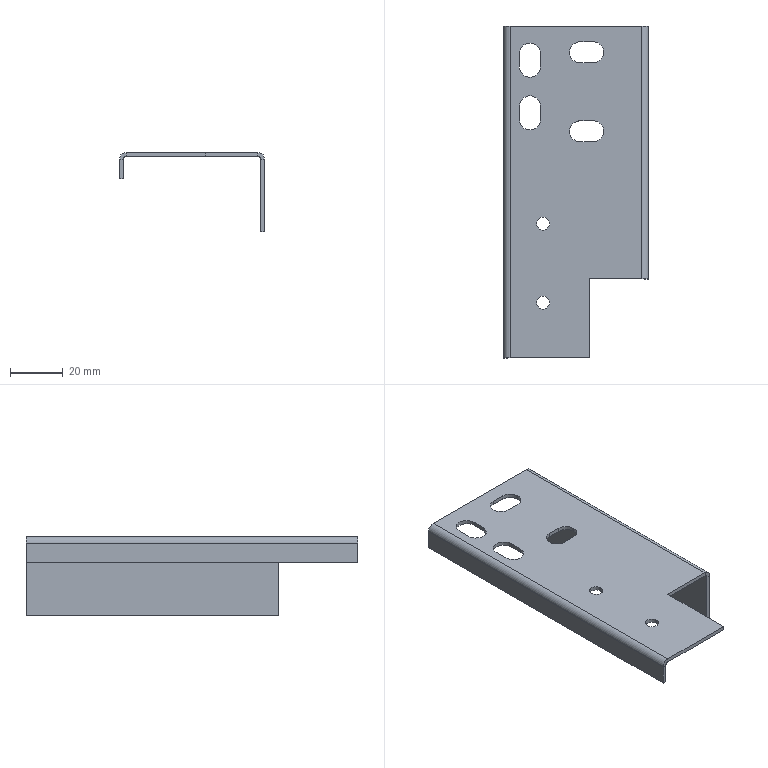Part | 1 solid | 46 faces | box 55 x 126 x 30 mm | volume 14242 mm3 | plane 28 | cylinder 18 | commonest cylinder face diameters 8 x10 5 x6 2 x2
STEP:
#1=CARTESIAN_POINT('',(10.5,53.,-1.5));
#2=VERTEX_POINT('',#1);
#3=CARTESIAN_POINT('',(6.5,57.,-1.5));
#4=VERTEX_POINT('',#3);
#5=CARTESIAN_POINT('',(6.5,53.,-1.5));
#6=DIRECTION('',(0.,0.,1.));
#7=DIRECTION('',(1.,0.,0.));
#8=AXIS2_PLACEMENT_3D('',#5,#6,#7);
#9=CIRCLE('',#8,4.);
#10=EDGE_CURVE('',#2,#4,#9,.T.);
#11=ORIENTED_EDGE('',*,*,#10,.F.);
#12=CARTESIAN_POINT('',(10.5,53.,0.));
#13=VERTEX_POINT('',#12);
#14=CARTESIAN_POINT('',(10.5,53.,-10.));
#15=DIRECTION('',(0.,0.,1.));
#16=VECTOR('',#15,1000.);
#17=LINE('',#14,#16);
#18=EDGE_CURVE('',#2,#13,#17,.T.);
#19=ORIENTED_EDGE('',*,*,#18,.T.);
#20=CARTESIAN_POINT('',(6.5,57.,0.));
#21=VERTEX_POINT('',#20);
#22=CARTESIAN_POINT('',(6.5,53.,0.));
#23=DIRECTION('',(0.,0.,1.));
#24=DIRECTION('',(1.,0.,0.));
#25=AXIS2_PLACEMENT_3D('',#22,#23,#24);
#26=CIRCLE('',#25,4.);
#27=EDGE_CURVE('',#13,#21,#26,.T.);
#28=ORIENTED_EDGE('',*,*,#27,.T.);
#29=CARTESIAN_POINT('',(6.5,57.,-10.));
#30=DIRECTION('',(0.,0.,1.));
#31=VECTOR('',#30,1000.);
#32=LINE('',#29,#31);
#33=EDGE_CURVE('',#4,#21,#32,.T.);
#34=ORIENTED_EDGE('',*,*,#33,.F.);
#35=EDGE_LOOP('',(#11,#19,#28,#34));
#36=FACE_OUTER_BOUND('',#35,.T.);
#37=CARTESIAN_POINT('',(6.5,53.,-10.));
#38=DIRECTION('',(0.,0.,1.));
#39=DIRECTION('',(1.,0.,0.));
#40=AXIS2_PLACEMENT_3D('',#37,#38,#39);
#41=CYLINDRICAL_SURFACE('',#40,4.);
#42=ADVANCED_FACE('',(#36),#41,.F.);
#43=CARTESIAN_POINT('',(10.5,23.,-1.5));
#44=VERTEX_POINT('',#43);
#45=CARTESIAN_POINT('',(6.5,27.,-1.5));
#46=VERTEX_POINT('',#45);
#47=CARTESIAN_POINT('',(6.5,23.,-1.5));
#48=DIRECTION('',(0.,0.,1.));
#49=DIRECTION('',(1.,0.,0.));
#50=AXIS2_PLACEMENT_3D('',#47,#48,#49);
#51=CIRCLE('',#50,4.);
#52=EDGE_CURVE('',#44,#46,#51,.T.);
#53=ORIENTED_EDGE('',*,*,#52,.F.);
#54=CARTESIAN_POINT('',(10.5,23.,0.));
#55=VERTEX_POINT('',#54);
#56=CARTESIAN_POINT('',(10.5,23.,-10.));
#57=DIRECTION('',(0.,0.,1.));
#58=VECTOR('',#57,1000.);
#59=LINE('',#56,#58);
#60=EDGE_CURVE('',#44,#55,#59,.T.);
#61=ORIENTED_EDGE('',*,*,#60,.T.);
#62=CARTESIAN_POINT('',(6.5,27.,0.));
#63=VERTEX_POINT('',#62);
#64=CARTESIAN_POINT('',(6.5,23.,0.));
#65=DIRECTION('',(0.,0.,1.));
#66=DIRECTION('',(1.,0.,0.));
#67=AXIS2_PLACEMENT_3D('',#64,#65,#66);
#68=CIRCLE('',#67,4.);
#69=EDGE_CURVE('',#55,#63,#68,.T.);
#70=ORIENTED_EDGE('',*,*,#69,.T.);
#71=CARTESIAN_POINT('',(6.5,27.,-10.));
#72=DIRECTION('',(0.,0.,1.));
#73=VECTOR('',#72,1000.);
#74=LINE('',#71,#73);
#75=EDGE_CURVE('',#46,#63,#74,.T.);
#76=ORIENTED_EDGE('',*,*,#75,.F.);
#77=EDGE_LOOP('',(#53,#61,#70,#76));
#78=FACE_OUTER_BOUND('',#77,.T.);
#79=CARTESIAN_POINT('',(6.5,23.,-10.));
#80=DIRECTION('',(0.,0.,1.));
#81=DIRECTION('',(1.,0.,0.));
#82=AXIS2_PLACEMENT_3D('',#79,#80,#81);
#83=CYLINDRICAL_SURFACE('',#82,4.);
#84=ADVANCED_FACE('',(#78),#83,.F.);
#85=CARTESIAN_POINT('',(-15.,-42.,-1.5));
#86=VERTEX_POINT('',#85);
#87=CARTESIAN_POINT('',(-10.,-42.,-1.5));
#88=VERTEX_POINT('',#87);
#89=CARTESIAN_POINT('',(-12.5,-42.,-1.5));
#90=DIRECTION('',(0.,0.,1.));
#91=DIRECTION('',(1.,0.,0.));
#92=AXIS2_PLACEMENT_3D('',#89,#90,#91);
#93=CIRCLE('',#92,2.5);
#94=EDGE_CURVE('',#86,#88,#93,.T.);
#95=ORIENTED_EDGE('',*,*,#94,.F.);
#96=CARTESIAN_POINT('',(-15.,-42.,0.));
#97=VERTEX_POINT('',#96);
#98=CARTESIAN_POINT('',(-15.,-42.,-10.));
#99=DIRECTION('',(0.,0.,1.));
#100=VECTOR('',#99,1000.);
#101=LINE('',#98,#100);
#102=EDGE_CURVE('',#86,#97,#101,.T.);
#103=ORIENTED_EDGE('',*,*,#102,.T.);
#104=CARTESIAN_POINT('',(-10.,-42.,0.));
#105=VERTEX_POINT('',#104);
#106=CARTESIAN_POINT('',(-12.5,-42.,0.));
#107=DIRECTION('',(0.,0.,1.));
#108=DIRECTION('',(1.,0.,0.));
#109=AXIS2_PLACEMENT_3D('',#106,#107,#108);
#110=CIRCLE('',#109,2.5);
#111=EDGE_CURVE('',#97,#105,#110,.T.);
#112=ORIENTED_EDGE('',*,*,#111,.T.);
#113=CARTESIAN_POINT('',(-10.,-42.,-10.));
#114=DIRECTION('',(0.,0.,1.));
#115=VECTOR('',#114,1000.);
#116=LINE('',#113,#115);
#117=EDGE_CURVE('',#88,#105,#116,.T.);
#118=ORIENTED_EDGE('',*,*,#117,.F.);
#119=EDGE_LOOP('',(#95,#103,#112,#118));
#120=FACE_OUTER_BOUND('',#119,.T.);
#121=CARTESIAN_POINT('',(-12.5,-42.,-10.));
#122=DIRECTION('',(0.,0.,1.));
#123=DIRECTION('',(1.,0.,0.));
#124=AXIS2_PLACEMENT_3D('',#121,#122,#123);
#125=CYLINDRICAL_SURFACE('',#124,2.5);
#126=ADVANCED_FACE('',(#120),#125,.F.);
#127=CARTESIAN_POINT('',(-15.,-12.,-1.5));
#128=VERTEX_POINT('',#127);
#129=CARTESIAN_POINT('',(-10.,-12.,-1.5));
#130=VERTEX_POINT('',#129);
#131=CARTESIAN_POINT('',(-12.5,-12.,-1.5));
#132=DIRECTION('',(0.,0.,1.));
#133=DIRECTION('',(1.,0.,0.));
#134=AXIS2_PLACEMENT_3D('',#131,#132,#133);
#135=CIRCLE('',#134,2.5);
#136=EDGE_CURVE('',#128,#130,#135,.T.);
#137=ORIENTED_EDGE('',*,*,#136,.F.);
#138=CARTESIAN_POINT('',(-15.,-12.,0.));
#139=VERTEX_POINT('',#138);
#140=CARTESIAN_POINT('',(-15.,-12.,-10.));
#141=DIRECTION('',(0.,0.,1.));
#142=VECTOR('',#141,1000.);
#143=LINE('',#140,#142);
#144=EDGE_CURVE('',#128,#139,#143,.T.);
#145=ORIENTED_EDGE('',*,*,#144,.T.);
#146=CARTESIAN_POINT('',(-10.,-12.,0.));
#147=VERTEX_POINT('',#146);
#148=CARTESIAN_POINT('',(-12.5,-12.,0.));
#149=DIRECTION('',(0.,0.,1.));
#150=DIRECTION('',(1.,0.,0.));
#151=AXIS2_PLACEMENT_3D('',#148,#149,#150);
#152=CIRCLE('',#151,2.5);
#153=EDGE_CURVE('',#139,#147,#152,.T.);
#154=ORIENTED_EDGE('',*,*,#153,.T.);
#155=CARTESIAN_POINT('',(-10.,-12.,-10.));
#156=DIRECTION('',(0.,0.,1.));
#157=VECTOR('',#156,1000.);
#158=LINE('',#155,#157);
#159=EDGE_CURVE('',#130,#147,#158,.T.);
#160=ORIENTED_EDGE('',*,*,#159,.F.);
#161=EDGE_LOOP('',(#137,#145,#154,#160));
#162=FACE_OUTER_BOUND('',#161,.T.);
#163=CARTESIAN_POINT('',(-12.5,-12.,-10.));
#164=DIRECTION('',(0.,0.,1.));
#165=DIRECTION('',(1.,0.,0.));
#166=AXIS2_PLACEMENT_3D('',#163,#164,#165);
#167=CYLINDRICAL_SURFACE('',#166,2.5);
#168=ADVANCED_FACE('',(#162),#167,.F.);
#169=CARTESIAN_POINT('',(27.5,-33.,-30.));
#170=VERTEX_POINT('',#169);
#171=CARTESIAN_POINT('',(27.5,-33.,-2.5));
#172=VERTEX_POINT('',#171);
#173=CARTESIAN_POINT('',(27.5,-33.,-30.));
#174=DIRECTION('',(0.,0.,1.));
#175=VECTOR('',#174,1000.);
#176=LINE('',#173,#175);
#177=EDGE_CURVE('',#170,#172,#176,.T.);
#178=ORIENTED_EDGE('',*,*,#177,.T.);
#179=CARTESIAN_POINT('',(26.,-33.,-2.5));
#180=VERTEX_POINT('',#179);
#181=CARTESIAN_POINT('',(27.5,-33.,-2.5));
#182=DIRECTION('',(-1.,0.,0.));
#183=VECTOR('',#182,1000.);
#184=LINE('',#181,#183);
#185=EDGE_CURVE('',#172,#180,#184,.T.);
#186=ORIENTED_EDGE('',*,*,#185,.T.);
#187=CARTESIAN_POINT('',(26.,-33.,-30.));
#188=VERTEX_POINT('',#187);
#189=CARTESIAN_POINT('',(26.,-33.,0.));
#190=DIRECTION('',(0.,0.,1.));
#191=VECTOR('',#190,1000.);
#192=LINE('',#189,#191);
#193=EDGE_CURVE('',#188,#180,#192,.T.);
#194=ORIENTED_EDGE('',*,*,#193,.F.);
#195=CARTESIAN_POINT('',(27.5,-33.,-30.));
#196=DIRECTION('',(-1.,0.,0.));
#197=VECTOR('',#196,1000.);
#198=LINE('',#195,#197);
#199=EDGE_CURVE('',#170,#188,#198,.T.);
#200=ORIENTED_EDGE('',*,*,#199,.F.);
#201=EDGE_LOOP('',(#178,#186,#194,#200));
#202=FACE_OUTER_BOUND('',#201,.T.);
#203=CARTESIAN_POINT('',(27.5,-33.,-30.));
#204=DIRECTION('',(0.,1.,0.));
#205=DIRECTION('',(0.,0.,1.));
#206=AXIS2_PLACEMENT_3D('',#203,#204,#205);
#207=PLANE('',#206);
#208=ADVANCED_FACE('',(#202),#207,.F.);
#209=CARTESIAN_POINT('',(25.,-33.,-1.5));
#210=VERTEX_POINT('',#209);
#211=CARTESIAN_POINT('',(5.,-33.,-1.5));
#212=VERTEX_POINT('',#211);
#213=CARTESIAN_POINT('',(0.,-33.,-1.5));
#214=DIRECTION('',(-1.,0.,0.));
#215=VECTOR('',#214,1000.);
#216=LINE('',#213,#215);
#217=EDGE_CURVE('',#210,#212,#216,.T.);
#218=ORIENTED_EDGE('',*,*,#217,.F.);
#219=CARTESIAN_POINT('',(25.,-33.,0.));
#220=VERTEX_POINT('',#219);
#221=CARTESIAN_POINT('',(25.,-33.,-1.5));
#222=DIRECTION('',(0.,0.,1.));
#223=VECTOR('',#222,1000.);
#224=LINE('',#221,#223);
#225=EDGE_CURVE('',#210,#220,#224,.T.);
#226=ORIENTED_EDGE('',*,*,#225,.T.);
#227=CARTESIAN_POINT('',(5.,-33.,0.));
#228=VERTEX_POINT('',#227);
#229=CARTESIAN_POINT('',(0.,-33.,0.));
#230=DIRECTION('',(-1.,0.,0.));
#231=VECTOR('',#230,1000.);
#232=LINE('',#229,#231);
#233=EDGE_CURVE('',#220,#228,#232,.T.);
#234=ORIENTED_EDGE('',*,*,#233,.T.);
#235=CARTESIAN_POINT('',(5.,-33.,-30.));
#236=DIRECTION('',(0.,0.,1.));
#237=VECTOR('',#236,1000.);
#238=LINE('',#235,#237);
#239=EDGE_CURVE('',#212,#228,#238,.T.);
#240=ORIENTED_EDGE('',*,*,#239,.F.);
#241=EDGE_LOOP('',(#218,#226,#234,#240));
#242=FACE_OUTER_BOUND('',#241,.T.);
#243=CARTESIAN_POINT('',(27.5,-33.,-30.));
#244=DIRECTION('',(0.,1.,0.));
#245=DIRECTION('',(0.,0.,1.));
#246=AXIS2_PLACEMENT_3D('',#243,#244,#245);
#247=PLANE('',#246);
#248=ADVANCED_FACE('',(#242),#247,.F.);
#249=CARTESIAN_POINT('',(-13.5,47.5,-1.5));
#250=VERTEX_POINT('',#249);
#251=CARTESIAN_POINT('',(-13.5,52.5,-1.5));
#252=VERTEX_POINT('',#251);
#253=CARTESIAN_POINT('',(-13.5,0.,-1.5));
#254=DIRECTION('',(0.,1.,0.));
#255=VECTOR('',#254,1000.);
#256=LINE('',#253,#255);
#257=EDGE_CURVE('',#250,#252,#256,.T.);
#258=ORIENTED_EDGE('',*,*,#257,.T.);
#259=CARTESIAN_POINT('',(-21.5,52.5,-1.5));
#260=VERTEX_POINT('',#259);
#261=CARTESIAN_POINT('',(-17.5,52.5,-1.5));
#262=DIRECTION('',(0.,0.,1.));
#263=DIRECTION('',(1.,0.,0.));
#264=AXIS2_PLACEMENT_3D('',#261,#262,#263);
#265=CIRCLE('',#264,4.);
#266=EDGE_CURVE('',#252,#260,#265,.T.);
#267=ORIENTED_EDGE('',*,*,#266,.T.);
#268=CARTESIAN_POINT('',(-21.5,47.5,-1.5));
#269=VERTEX_POINT('',#268);
#270=CARTESIAN_POINT('',(-21.5,0.,-1.5));
#271=DIRECTION('',(0.,-1.,0.));
#272=VECTOR('',#271,1000.);
#273=LINE('',#270,#272);
#274=EDGE_CURVE('',#260,#269,#273,.T.);
#275=ORIENTED_EDGE('',*,*,#274,.T.);
#276=CARTESIAN_POINT('',(-17.5,47.5,-1.5));
#277=DIRECTION('',(0.,0.,1.));
#278=DIRECTION('',(1.,0.,0.));
#279=AXIS2_PLACEMENT_3D('',#276,#277,#278);
#280=CIRCLE('',#279,4.);
#281=EDGE_CURVE('',#269,#250,#280,.T.);
#282=ORIENTED_EDGE('',*,*,#281,.T.);
#283=EDGE_LOOP('',(#258,#267,#275,#282));
#284=FACE_BOUND('',#283,.T.);
#285=CARTESIAN_POINT('',(-13.5,27.5,-1.5));
#286=VERTEX_POINT('',#285);
#287=CARTESIAN_POINT('',(-13.5,32.5,-1.5));
#288=VERTEX_POINT('',#287);
#289=CARTESIAN_POINT('',(-13.5,0.,-1.5));
#290=DIRECTION('',(0.,1.,0.));
#291=VECTOR('',#290,1000.);
#292=LINE('',#289,#291);
#293=EDGE_CURVE('',#286,#288,#292,.T.);
#294=ORIENTED_EDGE('',*,*,#293,.T.);
#295=CARTESIAN_POINT('',(-21.5,32.5,-1.5));
#296=VERTEX_POINT('',#295);
#297=CARTESIAN_POINT('',(-17.5,32.5,-1.5));
#298=DIRECTION('',(0.,0.,1.));
#299=DIRECTION('',(1.,0.,0.));
#300=AXIS2_PLACEMENT_3D('',#297,#298,#299);
#301=CIRCLE('',#300,4.);
#302=EDGE_CURVE('',#288,#296,#301,.T.);
#303=ORIENTED_EDGE('',*,*,#302,.T.);
#304=CARTESIAN_POINT('',(-21.5,27.5,-1.5));
#305=VERTEX_POINT('',#304);
#306=CARTESIAN_POINT('',(-21.5,0.,-1.5));
#307=DIRECTION('',(0.,-1.,0.));
#308=VECTOR('',#307,1000.);
#309=LINE('',#306,#308);
#310=EDGE_CURVE('',#296,#305,#309,.T.);
#311=ORIENTED_EDGE('',*,*,#310,.T.);
#312=CARTESIAN_POINT('',(-17.5,27.5,-1.5));
#313=DIRECTION('',(0.,0.,1.));
#314=DIRECTION('',(1.,0.,0.));
#315=AXIS2_PLACEMENT_3D('',#312,#313,#314);
#316=CIRCLE('',#315,4.);
#317=EDGE_CURVE('',#305,#286,#316,.T.);
#318=ORIENTED_EDGE('',*,*,#317,.T.);
#319=EDGE_LOOP('',(#294,#303,#311,#318));
#320=FACE_BOUND('',#319,.T.);
#321=CARTESIAN_POINT('',(1.5,57.,-1.5));
#322=VERTEX_POINT('',#321);
#323=CARTESIAN_POINT('',(0.,57.,-1.5));
#324=DIRECTION('',(-1.,0.,0.));
#325=VECTOR('',#324,1000.);
#326=LINE('',#323,#325);
#327=EDGE_CURVE('',#4,#322,#326,.T.);
#328=ORIENTED_EDGE('',*,*,#327,.T.);
#329=CARTESIAN_POINT('',(1.5,49.,-1.5));
#330=VERTEX_POINT('',#329);
#331=CARTESIAN_POINT('',(1.5,53.,-1.5));
#332=DIRECTION('',(0.,0.,1.));
#333=DIRECTION('',(1.,0.,0.));
#334=AXIS2_PLACEMENT_3D('',#331,#332,#333);
#335=CIRCLE('',#334,4.);
#336=EDGE_CURVE('',#322,#330,#335,.T.);
#337=ORIENTED_EDGE('',*,*,#336,.T.);
#338=CARTESIAN_POINT('',(6.5,49.,-1.5));
#339=VERTEX_POINT('',#338);
#340=CARTESIAN_POINT('',(0.,49.,-1.5));
#341=DIRECTION('',(1.,0.,0.));
#342=VECTOR('',#341,1000.);
#343=LINE('',#340,#342);
#344=EDGE_CURVE('',#330,#339,#343,.T.);
#345=ORIENTED_EDGE('',*,*,#344,.T.);
#346=CARTESIAN_POINT('',(6.5,53.,-1.5));
#347=DIRECTION('',(0.,0.,1.));
#348=DIRECTION('',(1.,0.,0.));
#349=AXIS2_PLACEMENT_3D('',#346,#347,#348);
#350=CIRCLE('',#349,4.);
#351=EDGE_CURVE('',#339,#2,#350,.T.);
#352=ORIENTED_EDGE('',*,*,#351,.T.);
#353=ORIENTED_EDGE('',*,*,#10,.T.);
#354=EDGE_LOOP('',(#328,#337,#345,#352,#353));
#355=FACE_BOUND('',#354,.T.);
#356=CARTESIAN_POINT('',(1.5,27.,-1.5));
#357=VERTEX_POINT('',#356);
#358=CARTESIAN_POINT('',(0.,27.,-1.5));
#359=DIRECTION('',(-1.,0.,0.));
#360=VECTOR('',#359,1000.);
#361=LINE('',#358,#360);
#362=EDGE_CURVE('',#46,#357,#361,.T.);
#363=ORIENTED_EDGE('',*,*,#362,.T.);
#364=CARTESIAN_POINT('',(1.5,19.,-1.5));
#365=VERTEX_POINT('',#364);
#366=CARTESIAN_POINT('',(1.5,23.,-1.5));
#367=DIRECTION('',(0.,0.,1.));
#368=DIRECTION('',(1.,0.,0.));
#369=AXIS2_PLACEMENT_3D('',#366,#367,#368);
#370=CIRCLE('',#369,4.);
#371=EDGE_CURVE('',#357,#365,#370,.T.);
#372=ORIENTED_EDGE('',*,*,#371,.T.);
#373=CARTESIAN_POINT('',(6.5,19.,-1.5));
#374=VERTEX_POINT('',#373);
#375=CARTESIAN_POINT('',(0.,19.,-1.5));
#376=DIRECTION('',(1.,0.,0.));
#377=VECTOR('',#376,1000.);
#378=LINE('',#375,#377);
#379=EDGE_CURVE('',#365,#374,#378,.T.);
#380=ORIENTED_EDGE('',*,*,#379,.T.);
#381=CARTESIAN_POINT('',(6.5,23.,-1.5));
#382=DIRECTION('',(0.,0.,1.));
#383=DIRECTION('',(1.,0.,0.));
#384=AXIS2_PLACEMENT_3D('',#381,#382,#383);
#385=CIRCLE('',#384,4.);
#386=EDGE_CURVE('',#374,#44,#385,.T.);
#387=ORIENTED_EDGE('',*,*,#386,.T.);
#388=ORIENTED_EDGE('',*,*,#52,.T.);
#389=EDGE_LOOP('',(#363,#372,#380,#387,#388));
#390=FACE_BOUND('',#389,.T.);
#391=CARTESIAN_POINT('',(-12.5,-42.,-1.5));
#392=DIRECTION('',(0.,0.,1.));
#393=DIRECTION('',(1.,0.,0.));
#394=AXIS2_PLACEMENT_3D('',#391,#392,#393);
#395=CIRCLE('',#394,2.5);
#396=EDGE_CURVE('',#88,#86,#395,.T.);
#397=ORIENTED_EDGE('',*,*,#396,.T.);
#398=ORIENTED_EDGE('',*,*,#94,.T.);
#399=EDGE_LOOP('',(#397,#398));
#400=FACE_BOUND('',#399,.T.);
#401=CARTESIAN_POINT('',(-12.5,-12.,-1.5));
#402=DIRECTION('',(0.,0.,1.));
#403=DIRECTION('',(1.,0.,0.));
#404=AXIS2_PLACEMENT_3D('',#401,#402,#403);
#405=CIRCLE('',#404,2.5);
#406=EDGE_CURVE('',#130,#128,#405,.T.);
#407=ORIENTED_EDGE('',*,*,#406,.T.);
#408=ORIENTED_EDGE('',*,*,#136,.T.);
#409=EDGE_LOOP('',(#407,#408));
#410=FACE_BOUND('',#409,.T.);
#411=ORIENTED_EDGE('',*,*,#217,.T.);
#412=CARTESIAN_POINT('',(5.,-63.,-1.5));
#413=VERTEX_POINT('',#412);
#414=CARTESIAN_POINT('',(5.,0.,-1.5));
#415=DIRECTION('',(0.,-1.,0.));
#416=VECTOR('',#415,1000.);
#417=LINE('',#414,#416);
#418=EDGE_CURVE('',#212,#413,#417,.T.);
#419=ORIENTED_EDGE('',*,*,#418,.T.);
#420=CARTESIAN_POINT('',(-25.,-63.,-1.5));
#421=VERTEX_POINT('',#420);
#422=CARTESIAN_POINT('',(-27.5,-63.,-1.5));
#423=DIRECTION('',(1.,0.,0.));
#424=VECTOR('',#423,1000.);
#425=LINE('',#422,#424);
#426=EDGE_CURVE('',#421,#413,#425,.T.);
#427=ORIENTED_EDGE('',*,*,#426,.F.);
#428=CARTESIAN_POINT('',(-25.,63.,-1.5));
#429=VERTEX_POINT('',#428);
#430=CARTESIAN_POINT('',(-25.,63.,-1.5));
#431=DIRECTION('',(0.,-1.,0.));
#432=VECTOR('',#431,1000.);
#433=LINE('',#430,#432);
#434=EDGE_CURVE('',#429,#421,#433,.T.);
#435=ORIENTED_EDGE('',*,*,#434,.F.);
#436=CARTESIAN_POINT('',(25.,63.,-1.5));
#437=VERTEX_POINT('',#436);
#438=CARTESIAN_POINT('',(-27.5,63.,-1.5));
#439=DIRECTION('',(-1.,0.,0.));
#440=VECTOR('',#439,1000.);
#441=LINE('',#438,#440);
#442=EDGE_CURVE('',#437,#429,#441,.T.);
#443=ORIENTED_EDGE('',*,*,#442,.F.);
#444=CARTESIAN_POINT('',(25.,-63.,-1.5));
#445=DIRECTION('',(0.,1.,0.));
#446=VECTOR('',#445,1000.);
#447=LINE('',#444,#446);
#448=EDGE_CURVE('',#210,#437,#447,.T.);
#449=ORIENTED_EDGE('',*,*,#448,.F.);
#450=EDGE_LOOP('',(#411,#419,#427,#435,#443,#449));
#451=FACE_OUTER_BOUND('',#450,.T.);
#452=CARTESIAN_POINT('',(0.,0.,-1.5));
#453=DIRECTION('',(0.,0.,1.));
#454=DIRECTION('',(1.,0.,0.));
#455=AXIS2_PLACEMENT_3D('',#452,#453,#454);
#456=PLANE('',#455);
#457=ADVANCED_FACE('',(#284,#320,#355,#390,#400,#410,#451),#456,.F.);
#458=CARTESIAN_POINT('',(-13.5,52.5,0.));
#459=VERTEX_POINT('',#458);
#460=CARTESIAN_POINT('',(-21.5,52.5,0.));
#461=VERTEX_POINT('',#460);
#462=CARTESIAN_POINT('',(-17.5,52.5,0.));
#463=DIRECTION('',(0.,0.,1.));
#464=DIRECTION('',(1.,0.,0.));
#465=AXIS2_PLACEMENT_3D('',#462,#463,#464);
#466=CIRCLE('',#465,4.);
#467=EDGE_CURVE('',#459,#461,#466,.T.);
#468=ORIENTED_EDGE('',*,*,#467,.F.);
#469=CARTESIAN_POINT('',(-13.5,47.5,0.));
#470=VERTEX_POINT('',#469);
#471=CARTESIAN_POINT('',(-13.5,52.5,0.));
#472=DIRECTION('',(0.,1.,0.));
#473=VECTOR('',#472,1000.);
#474=LINE('',#471,#473);
#475=EDGE_CURVE('',#470,#459,#474,.T.);
#476=ORIENTED_EDGE('',*,*,#475,.F.);
#477=CARTESIAN_POINT('',(-21.5,47.5,0.));
#478=VERTEX_POINT('',#477);
#479=CARTESIAN_POINT('',(-17.5,47.5,0.));
#480=DIRECTION('',(0.,0.,1.));
#481=DIRECTION('',(1.,0.,0.));
#482=AXIS2_PLACEMENT_3D('',#479,#480,#481);
#483=CIRCLE('',#482,4.);
#484=EDGE_CURVE('',#478,#470,#483,.T.);
#485=ORIENTED_EDGE('',*,*,#484,.F.);
#486=CARTESIAN_POINT('',(-21.5,52.5,0.));
#487=DIRECTION('',(0.,-1.,0.));
#488=VECTOR('',#487,1000.);
#489=LINE('',#486,#488);
#490=EDGE_CURVE('',#461,#478,#489,.T.);
#491=ORIENTED_EDGE('',*,*,#490,.F.);
#492=EDGE_LOOP('',(#468,#476,#485,#491));
#493=FACE_BOUND('',#492,.T.);
#494=CARTESIAN_POINT('',(-13.5,32.5,0.));
#495=VERTEX_POINT('',#494);
#496=CARTESIAN_POINT('',(-21.5,32.5,0.));
#497=VERTEX_POINT('',#496);
#498=CARTESIAN_POINT('',(-17.5,32.5,0.));
#499=DIRECTION('',(0.,0.,1.));
#500=DIRECTION('',(1.,0.,0.));
#501=AXIS2_PLACEMENT_3D('',#498,#499,#500);
#502=CIRCLE('',#501,4.);
#503=EDGE_CURVE('',#495,#497,#502,.T.);
#504=ORIENTED_EDGE('',*,*,#503,.F.);
#505=CARTESIAN_POINT('',(-13.5,27.5,0.));
#506=VERTEX_POINT('',#505);
#507=CARTESIAN_POINT('',(-13.5,32.5,0.));
#508=DIRECTION('',(0.,1.,0.));
#509=VECTOR('',#508,1000.);
#510=LINE('',#507,#509);
#511=EDGE_CURVE('',#506,#495,#510,.T.);
#512=ORIENTED_EDGE('',*,*,#511,.F.);
#513=CARTESIAN_POINT('',(-21.5,27.5,0.));
#514=VERTEX_POINT('',#513);
#515=CARTESIAN_POINT('',(-17.5,27.5,0.));
#516=DIRECTION('',(0.,0.,1.));
#517=DIRECTION('',(1.,0.,0.));
#518=AXIS2_PLACEMENT_3D('',#515,#516,#517);
#519=CIRCLE('',#518,4.);
#520=EDGE_CURVE('',#514,#506,#519,.T.);
#521=ORIENTED_EDGE('',*,*,#520,.F.);
#522=CARTESIAN_POINT('',(-21.5,32.5,0.));
#523=DIRECTION('',(0.,-1.,0.));
#524=VECTOR('',#523,1000.);
#525=LINE('',#522,#524);
#526=EDGE_CURVE('',#497,#514,#525,.T.);
#527=ORIENTED_EDGE('',*,*,#526,.F.);
#528=EDGE_LOOP('',(#504,#512,#521,#527));
#529=FACE_BOUND('',#528,.T.);
#530=CARTESIAN_POINT('',(1.5,57.,0.));
#531=VERTEX_POINT('',#530);
#532=CARTESIAN_POINT('',(1.5,49.,0.));
#533=VERTEX_POINT('',#532);
#534=CARTESIAN_POINT('',(1.5,53.,0.));
#535=DIRECTION('',(0.,0.,1.));
#536=DIRECTION('',(1.,0.,0.));
#537=AXIS2_PLACEMENT_3D('',#534,#535,#536);
#538=CIRCLE('',#537,4.);
#539=EDGE_CURVE('',#531,#533,#538,.T.);
#540=ORIENTED_EDGE('',*,*,#539,.F.);
#541=CARTESIAN_POINT('',(1.5,57.,0.));
#542=DIRECTION('',(-1.,0.,0.));
#543=VECTOR('',#542,1000.);
#544=LINE('',#541,#543);
#545=EDGE_CURVE('',#21,#531,#544,.T.);
#546=ORIENTED_EDGE('',*,*,#545,.F.);
#547=ORIENTED_EDGE('',*,*,#27,.F.);
#548=CARTESIAN_POINT('',(6.5,49.,0.));
#549=VERTEX_POINT('',#548);
#550=CARTESIAN_POINT('',(6.5,53.,0.));
#551=DIRECTION('',(0.,0.,1.));
#552=DIRECTION('',(1.,0.,0.));
#553=AXIS2_PLACEMENT_3D('',#550,#551,#552);
#554=CIRCLE('',#553,4.);
#555=EDGE_CURVE('',#549,#13,#554,.T.);
#556=ORIENTED_EDGE('',*,*,#555,.F.);
#557=CARTESIAN_POINT('',(1.5,49.,0.));
#558=DIRECTION('',(1.,0.,0.));
#559=VECTOR('',#558,1000.);
#560=LINE('',#557,#559);
#561=EDGE_CURVE('',#533,#549,#560,.T.);
#562=ORIENTED_EDGE('',*,*,#561,.F.);
#563=EDGE_LOOP('',(#540,#546,#547,#556,#562));
#564=FACE_BOUND('',#563,.T.);
#565=CARTESIAN_POINT('',(1.5,27.,0.));
#566=VERTEX_POINT('',#565);
#567=CARTESIAN_POINT('',(1.5,19.,0.));
#568=VERTEX_POINT('',#567);
#569=CARTESIAN_POINT('',(1.5,23.,0.));
#570=DIRECTION('',(0.,0.,1.));
#571=DIRECTION('',(1.,0.,0.));
#572=AXIS2_PLACEMENT_3D('',#569,#570,#571);
#573=CIRCLE('',#572,4.);
#574=EDGE_CURVE('',#566,#568,#573,.T.);
#575=ORIENTED_EDGE('',*,*,#574,.F.);
#576=CARTESIAN_POINT('',(1.5,27.,0.));
#577=DIRECTION('',(-1.,0.,0.));
#578=VECTOR('',#577,1000.);
#579=LINE('',#576,#578);
#580=EDGE_CURVE('',#63,#566,#579,.T.);
#581=ORIENTED_EDGE('',*,*,#580,.F.);
#582=ORIENTED_EDGE('',*,*,#69,.F.);
#583=CARTESIAN_POINT('',(6.5,19.,0.));
#584=VERTEX_POINT('',#583);
#585=CARTESIAN_POINT('',(6.5,23.,0.));
#586=DIRECTION('',(0.,0.,1.));
#587=DIRECTION('',(1.,0.,0.));
#588=AXIS2_PLACEMENT_3D('',#585,#586,#587);
#589=CIRCLE('',#588,4.);
#590=EDGE_CURVE('',#584,#55,#589,.T.);
#591=ORIENTED_EDGE('',*,*,#590,.F.);
#592=CARTESIAN_POINT('',(1.5,19.,0.));
#593=DIRECTION('',(1.,0.,0.));
#594=VECTOR('',#593,1000.);
#595=LINE('',#592,#594);
#596=EDGE_CURVE('',#568,#584,#595,.T.);
#597=ORIENTED_EDGE('',*,*,#596,.F.);
#598=EDGE_LOOP('',(#575,#581,#582,#591,#597));
#599=FACE_BOUND('',#598,.T.);
#600=CARTESIAN_POINT('',(-12.5,-42.,0.));
#601=DIRECTION('',(0.,0.,1.));
#602=DIRECTION('',(1.,0.,0.));
#603=AXIS2_PLACEMENT_3D('',#600,#601,#602);
#604=CIRCLE('',#603,2.5);
#605=EDGE_CURVE('',#105,#97,#604,.T.);
#606=ORIENTED_EDGE('',*,*,#605,.F.);
#607=ORIENTED_EDGE('',*,*,#111,.F.);
#608=EDGE_LOOP('',(#606,#607));
#609=FACE_BOUND('',#608,.T.);
#610=CARTESIAN_POINT('',(-12.5,-12.,0.));
#611=DIRECTION('',(0.,0.,1.));
#612=DIRECTION('',(1.,0.,0.));
#613=AXIS2_PLACEMENT_3D('',#610,#611,#612);
#614=CIRCLE('',#613,2.5);
#615=EDGE_CURVE('',#147,#139,#614,.T.);
#616=ORIENTED_EDGE('',*,*,#615,.F.);
#617=ORIENTED_EDGE('',*,*,#153,.F.);
#618=EDGE_LOOP('',(#616,#617));
#619=FACE_BOUND('',#618,.T.);
#620=CARTESIAN_POINT('',(5.,-63.,0.));
#621=VERTEX_POINT('',#620);
#622=CARTESIAN_POINT('',(5.,0.,0.));
#623=DIRECTION('',(0.,-1.,0.));
#624=VECTOR('',#623,1000.);
#625=LINE('',#622,#624);
#626=EDGE_CURVE('',#228,#621,#625,.T.);
#627=ORIENTED_EDGE('',*,*,#626,.F.);
#628=ORIENTED_EDGE('',*,*,#233,.F.);
#629=CARTESIAN_POINT('',(25.,63.,0.));
#630=VERTEX_POINT('',#629);
#631=CARTESIAN_POINT('',(25.,-63.,0.));
#632=DIRECTION('',(0.,1.,0.));
#633=VECTOR('',#632,1000.);
#634=LINE('',#631,#633);
#635=EDGE_CURVE('',#220,#630,#634,.T.);
#636=ORIENTED_EDGE('',*,*,#635,.T.);
#637=CARTESIAN_POINT('',(-25.,63.,0.));
#638=VERTEX_POINT('',#637);
#639=CARTESIAN_POINT('',(-27.5,63.,0.));
#640=DIRECTION('',(-1.,0.,0.));
#641=VECTOR('',#640,1000.);
#642=LINE('',#639,#641);
#643=EDGE_CURVE('',#630,#638,#642,.T.);
#644=ORIENTED_EDGE('',*,*,#643,.T.);
#645=CARTESIAN_POINT('',(-25.,-63.,0.));
#646=VERTEX_POINT('',#645);
#647=CARTESIAN_POINT('',(-25.,63.,0.));
#648=DIRECTION('',(0.,-1.,0.));
#649=VECTOR('',#648,1000.);
#650=LINE('',#647,#649);
#651=EDGE_CURVE('',#638,#646,#650,.T.);
#652=ORIENTED_EDGE('',*,*,#651,.T.);
#653=CARTESIAN_POINT('',(-27.5,-63.,0.));
#654=DIRECTION('',(1.,0.,0.));
#655=VECTOR('',#654,1000.);
#656=LINE('',#653,#655);
#657=EDGE_CURVE('',#646,#621,#656,.T.);
#658=ORIENTED_EDGE('',*,*,#657,.T.);
#659=EDGE_LOOP('',(#627,#628,#636,#644,#652,#658));
#660=FACE_OUTER_BOUND('',#659,.T.);
#661=CARTESIAN_POINT('',(0.,0.,0.));
#662=DIRECTION('',(0.,0.,1.));
#663=DIRECTION('',(1.,0.,0.));
#664=AXIS2_PLACEMENT_3D('',#661,#662,#663);
#665=PLANE('',#664);
#666=ADVANCED_FACE('',(#493,#529,#564,#599,#609,#619,#660),#665,.T.);
#667=ORIENTED_EDGE('',*,*,#442,.T.);
#668=CARTESIAN_POINT('',(-25.,63.,-1.5));
#669=DIRECTION('',(0.,0.,1.));
#670=VECTOR('',#669,1000.);
#671=LINE('',#668,#670);
#672=EDGE_CURVE('',#429,#638,#671,.T.);
#673=ORIENTED_EDGE('',*,*,#672,.T.);
#674=ORIENTED_EDGE('',*,*,#643,.F.);
#675=CARTESIAN_POINT('',(25.,63.,-1.5));
#676=DIRECTION('',(0.,0.,1.));
#677=VECTOR('',#676,1000.);
#678=LINE('',#675,#677);
#679=EDGE_CURVE('',#437,#630,#678,.T.);
#680=ORIENTED_EDGE('',*,*,#679,.F.);
#681=EDGE_LOOP('',(#667,#673,#674,#680));
#682=FACE_OUTER_BOUND('',#681,.T.);
#683=CARTESIAN_POINT('',(-27.5,63.,-1.5));
#684=DIRECTION('',(0.,1.,0.));
#685=DIRECTION('',(0.,0.,1.));
#686=AXIS2_PLACEMENT_3D('',#683,#684,#685);
#687=PLANE('',#686);
#688=ADVANCED_FACE('',(#682),#687,.T.);
#689=CARTESIAN_POINT('',(5.,-63.,-30.));
#690=DIRECTION('',(0.,0.,1.));
#691=VECTOR('',#690,1000.);
#692=LINE('',#689,#691);
#693=EDGE_CURVE('',#413,#621,#692,.T.);
#694=ORIENTED_EDGE('',*,*,#693,.T.);
#695=ORIENTED_EDGE('',*,*,#657,.F.);
#696=CARTESIAN_POINT('',(-25.,-63.,-1.5));
#697=DIRECTION('',(0.,0.,1.));
#698=VECTOR('',#697,1000.);
#699=LINE('',#696,#698);
#700=EDGE_CURVE('',#421,#646,#699,.T.);
#701=ORIENTED_EDGE('',*,*,#700,.F.);
#702=ORIENTED_EDGE('',*,*,#426,.T.);
#703=EDGE_LOOP('',(#694,#695,#701,#702));
#704=FACE_OUTER_BOUND('',#703,.T.);
#705=CARTESIAN_POINT('',(-27.5,-63.,-1.5));
#706=DIRECTION('',(0.,-1.,0.));
#707=DIRECTION('',(0.,0.,-1.));
#708=AXIS2_PLACEMENT_3D('',#705,#706,#707);
#709=PLANE('',#708);
#710=ADVANCED_FACE('',(#704),#709,.T.);
#711=CARTESIAN_POINT('',(26.,63.,-2.5));
#712=VERTEX_POINT('',#711);
#713=CARTESIAN_POINT('',(27.5,63.,-2.5));
#714=VERTEX_POINT('',#713);
#715=CARTESIAN_POINT('',(27.5,63.,-2.5));
#716=DIRECTION('',(1.,0.,0.));
#717=VECTOR('',#716,1000.);
#718=LINE('',#715,#717);
#719=EDGE_CURVE('',#712,#714,#718,.T.);
#720=ORIENTED_EDGE('',*,*,#719,.F.);
#721=CARTESIAN_POINT('',(25.,63.,-2.5));
#722=DIRECTION('',(0.,1.,0.));
#723=DIRECTION('',(0.,0.,-1.));
#724=AXIS2_PLACEMENT_3D('',#721,#722,#723);
#725=CIRCLE('',#724,1.);
#726=EDGE_CURVE('',#437,#712,#725,.T.);
#727=ORIENTED_EDGE('',*,*,#726,.F.);
#728=ORIENTED_EDGE('',*,*,#679,.T.);
#729=CARTESIAN_POINT('',(25.,63.,-2.5));
#730=DIRECTION('',(0.,1.,0.));
#731=DIRECTION('',(0.,0.,-1.));
#732=AXIS2_PLACEMENT_3D('',#729,#730,#731);
#733=CIRCLE('',#732,2.5);
#734=EDGE_CURVE('',#630,#714,#733,.T.);
#735=ORIENTED_EDGE('',*,*,#734,.T.);
#736=EDGE_LOOP('',(#720,#727,#728,#735));
#737=FACE_OUTER_BOUND('',#736,.T.);
#738=CARTESIAN_POINT('',(25.,63.,-2.5));
#739=DIRECTION('',(0.,1.,0.));
#740=DIRECTION('',(0.,0.,1.));
#741=AXIS2_PLACEMENT_3D('',#738,#739,#740);
#742=PLANE('',#741);
#743=ADVANCED_FACE('',(#737),#742,.T.);
#744=CARTESIAN_POINT('',(25.,-33.,-2.5));
#745=DIRECTION('',(0.,-1.,0.));
#746=DIRECTION('',(0.,0.,1.));
#747=AXIS2_PLACEMENT_3D('',#744,#745,#746);
#748=CIRCLE('',#747,2.5);
#749=EDGE_CURVE('',#172,#220,#748,.T.);
#750=ORIENTED_EDGE('',*,*,#749,.F.);
#751=CARTESIAN_POINT('',(27.5,0.,-2.5));
#752=DIRECTION('',(0.,-1.,0.));
#753=VECTOR('',#752,1000.);
#754=LINE('',#751,#753);
#755=EDGE_CURVE('',#714,#172,#754,.T.);
#756=ORIENTED_EDGE('',*,*,#755,.F.);
#757=ORIENTED_EDGE('',*,*,#734,.F.);
#758=ORIENTED_EDGE('',*,*,#635,.F.);
#759=EDGE_LOOP('',(#750,#756,#757,#758));
#760=FACE_OUTER_BOUND('',#759,.T.);
#761=CARTESIAN_POINT('',(25.,-63.,-2.5));
#762=DIRECTION('',(0.,-1.,0.));
#763=DIRECTION('',(1.,0.,0.));
#764=AXIS2_PLACEMENT_3D('',#761,#762,#763);
#765=CYLINDRICAL_SURFACE('',#764,2.5);
#766=ADVANCED_FACE('',(#760),#765,.T.);
#767=CARTESIAN_POINT('',(26.,63.,-2.5));
#768=DIRECTION('',(0.,-1.,0.));
#769=VECTOR('',#768,1000.);
#770=LINE('',#767,#769);
#771=EDGE_CURVE('',#712,#180,#770,.T.);
#772=ORIENTED_EDGE('',*,*,#771,.T.);
#773=CARTESIAN_POINT('',(25.,-33.,-2.5));
#774=DIRECTION('',(0.,-1.,0.));
#775=DIRECTION('',(0.,0.,1.));
#776=AXIS2_PLACEMENT_3D('',#773,#774,#775);
#777=CIRCLE('',#776,1.);
#778=EDGE_CURVE('',#180,#210,#777,.T.);
#779=ORIENTED_EDGE('',*,*,#778,.T.);
#780=ORIENTED_EDGE('',*,*,#448,.T.);
#781=ORIENTED_EDGE('',*,*,#726,.T.);
#782=EDGE_LOOP('',(#772,#779,#780,#781));
#783=FACE_OUTER_BOUND('',#782,.T.);
#784=CARTESIAN_POINT('',(25.,-63.,-2.5));
#785=DIRECTION('',(0.,-1.,0.));
#786=DIRECTION('',(1.,0.,0.));
#787=AXIS2_PLACEMENT_3D('',#784,#785,#786);
#788=CYLINDRICAL_SURFACE('',#787,1.);
#789=ADVANCED_FACE('',(#783),#788,.F.);
#790=CARTESIAN_POINT('',(26.,63.,-30.));
#791=VERTEX_POINT('',#790);
#792=CARTESIAN_POINT('',(26.,63.,0.));
#793=DIRECTION('',(0.,0.,-1.));
#794=VECTOR('',#793,1000.);
#795=LINE('',#792,#794);
#796=EDGE_CURVE('',#712,#791,#795,.T.);
#797=ORIENTED_EDGE('',*,*,#796,.F.);
#798=ORIENTED_EDGE('',*,*,#719,.T.);
#799=CARTESIAN_POINT('',(27.5,63.,-30.));
#800=VERTEX_POINT('',#799);
#801=CARTESIAN_POINT('',(27.5,63.,-30.));
#802=DIRECTION('',(0.,0.,-1.));
#803=VECTOR('',#802,1000.);
#804=LINE('',#801,#803);
#805=EDGE_CURVE('',#714,#800,#804,.T.);
#806=ORIENTED_EDGE('',*,*,#805,.T.);
#807=CARTESIAN_POINT('',(27.5,63.,-30.));
#808=DIRECTION('',(-1.,0.,0.));
#809=VECTOR('',#808,1000.);
#810=LINE('',#807,#809);
#811=EDGE_CURVE('',#800,#791,#810,.T.);
#812=ORIENTED_EDGE('',*,*,#811,.T.);
#813=EDGE_LOOP('',(#797,#798,#806,#812));
#814=FACE_OUTER_BOUND('',#813,.T.);
#815=CARTESIAN_POINT('',(27.5,63.,-30.));
#816=DIRECTION('',(0.,1.,0.));
#817=DIRECTION('',(-1.,0.,0.));
#818=AXIS2_PLACEMENT_3D('',#815,#816,#817);
#819=PLANE('',#818);
#820=ADVANCED_FACE('',(#814),#819,.T.);
#821=ORIENTED_EDGE('',*,*,#177,.F.);
#822=CARTESIAN_POINT('',(27.5,-63.,-30.));
#823=DIRECTION('',(0.,-1.,0.));
#824=VECTOR('',#823,1000.);
#825=LINE('',#822,#824);
#826=EDGE_CURVE('',#800,#170,#825,.T.);
#827=ORIENTED_EDGE('',*,*,#826,.F.);
#828=ORIENTED_EDGE('',*,*,#805,.F.);
#829=ORIENTED_EDGE('',*,*,#755,.T.);
#830=EDGE_LOOP('',(#821,#827,#828,#829));
#831=FACE_OUTER_BOUND('',#830,.T.);
#832=CARTESIAN_POINT('',(27.5,0.,0.));
#833=DIRECTION('',(1.,0.,0.));
#834=DIRECTION('',(0.,0.,-1.));
#835=AXIS2_PLACEMENT_3D('',#832,#833,#834);
#836=PLANE('',#835);
#837=ADVANCED_FACE('',(#831),#836,.T.);
#838=CARTESIAN_POINT('',(26.,0.,-30.));
#839=DIRECTION('',(0.,-1.,0.));
#840=VECTOR('',#839,1000.);
#841=LINE('',#838,#840);
#842=EDGE_CURVE('',#791,#188,#841,.T.);
#843=ORIENTED_EDGE('',*,*,#842,.T.);
#844=ORIENTED_EDGE('',*,*,#193,.T.);
#845=ORIENTED_EDGE('',*,*,#771,.F.);
#846=ORIENTED_EDGE('',*,*,#796,.T.);
#847=EDGE_LOOP('',(#843,#844,#845,#846));
#848=FACE_OUTER_BOUND('',#847,.T.);
#849=CARTESIAN_POINT('',(26.,0.,0.));
#850=DIRECTION('',(1.,0.,0.));
#851=DIRECTION('',(0.,0.,-1.));
#852=AXIS2_PLACEMENT_3D('',#849,#850,#851);
#853=PLANE('',#852);
#854=ADVANCED_FACE('',(#848),#853,.F.);
#855=ORIENTED_EDGE('',*,*,#199,.T.);
#856=ORIENTED_EDGE('',*,*,#842,.F.);
#857=ORIENTED_EDGE('',*,*,#811,.F.);
#858=ORIENTED_EDGE('',*,*,#826,.T.);
#859=EDGE_LOOP('',(#855,#856,#857,#858));
#860=FACE_OUTER_BOUND('',#859,.T.);
#861=CARTESIAN_POINT('',(27.5,-63.,-30.));
#862=DIRECTION('',(0.,0.,-1.));
#863=DIRECTION('',(-1.,0.,0.));
#864=AXIS2_PLACEMENT_3D('',#861,#862,#863);
#865=PLANE('',#864);
#866=ADVANCED_FACE('',(#860),#865,.T.);
#867=CARTESIAN_POINT('',(-26.,-63.,-2.5));
#868=VERTEX_POINT('',#867);
#869=CARTESIAN_POINT('',(-27.5,-63.,-2.5));
#870=VERTEX_POINT('',#869);
#871=CARTESIAN_POINT('',(-27.5,-63.,-2.5));
#872=DIRECTION('',(-1.,0.,0.));
#873=VECTOR('',#872,1000.);
#874=LINE('',#871,#873);
#875=EDGE_CURVE('',#868,#870,#874,.T.);
#876=ORIENTED_EDGE('',*,*,#875,.F.);
#877=CARTESIAN_POINT('',(-25.,-63.,-2.5));
#878=DIRECTION('',(0.,-1.,0.));
#879=DIRECTION('',(0.,0.,1.));
#880=AXIS2_PLACEMENT_3D('',#877,#878,#879);
#881=CIRCLE('',#880,1.);
#882=EDGE_CURVE('',#421,#868,#881,.T.);
#883=ORIENTED_EDGE('',*,*,#882,.F.);
#884=ORIENTED_EDGE('',*,*,#700,.T.);
#885=CARTESIAN_POINT('',(-25.,-63.,-2.5));
#886=DIRECTION('',(0.,-1.,0.));
#887=DIRECTION('',(0.,0.,1.));
#888=AXIS2_PLACEMENT_3D('',#885,#886,#887);
#889=CIRCLE('',#888,2.5);
#890=EDGE_CURVE('',#646,#870,#889,.T.);
#891=ORIENTED_EDGE('',*,*,#890,.T.);
#892=EDGE_LOOP('',(#876,#883,#884,#891));
#893=FACE_OUTER_BOUND('',#892,.T.);
#894=CARTESIAN_POINT('',(-25.,-63.,-2.5));
#895=DIRECTION('',(0.,-1.,0.));
#896=DIRECTION('',(0.,0.,-1.));
#897=AXIS2_PLACEMENT_3D('',#894,#895,#896);
#898=PLANE('',#897);
#899=ADVANCED_FACE('',(#893),#898,.T.);
#900=CARTESIAN_POINT('',(-26.,63.,-2.5));
#901=VERTEX_POINT('',#900);
#902=CARTESIAN_POINT('',(-25.,63.,-2.5));
#903=DIRECTION('',(0.,1.,0.));
#904=DIRECTION('',(0.,0.,1.));
#905=AXIS2_PLACEMENT_3D('',#902,#903,#904);
#906=CIRCLE('',#905,1.);
#907=EDGE_CURVE('',#901,#429,#906,.T.);
#908=ORIENTED_EDGE('',*,*,#907,.F.);
#909=CARTESIAN_POINT('',(-27.5,63.,-2.5));
#910=VERTEX_POINT('',#909);
#911=CARTESIAN_POINT('',(-26.,63.,-2.5));
#912=DIRECTION('',(-1.,0.,0.));
#913=VECTOR('',#912,1000.);
#914=LINE('',#911,#913);
#915=EDGE_CURVE('',#901,#910,#914,.T.);
#916=ORIENTED_EDGE('',*,*,#915,.T.);
#917=CARTESIAN_POINT('',(-25.,63.,-2.5));
#918=DIRECTION('',(0.,1.,0.));
#919=DIRECTION('',(0.,0.,1.));
#920=AXIS2_PLACEMENT_3D('',#917,#918,#919);
#921=CIRCLE('',#920,2.5);
#922=EDGE_CURVE('',#910,#638,#921,.T.);
#923=ORIENTED_EDGE('',*,*,#922,.T.);
#924=ORIENTED_EDGE('',*,*,#672,.F.);
#925=EDGE_LOOP('',(#908,#916,#923,#924));
#926=FACE_OUTER_BOUND('',#925,.T.);
#927=CARTESIAN_POINT('',(-25.,63.,-2.5));
#928=DIRECTION('',(0.,-1.,0.));
#929=DIRECTION('',(0.,0.,-1.));
#930=AXIS2_PLACEMENT_3D('',#927,#928,#929);
#931=PLANE('',#930);
#932=ADVANCED_FACE('',(#926),#931,.F.);
#933=ORIENTED_EDGE('',*,*,#651,.F.);
#934=ORIENTED_EDGE('',*,*,#922,.F.);
#935=CARTESIAN_POINT('',(-27.5,0.,-2.5));
#936=DIRECTION('',(0.,1.,0.));
#937=VECTOR('',#936,1000.);
#938=LINE('',#935,#937);
#939=EDGE_CURVE('',#870,#910,#938,.T.);
#940=ORIENTED_EDGE('',*,*,#939,.F.);
#941=ORIENTED_EDGE('',*,*,#890,.F.);
#942=EDGE_LOOP('',(#933,#934,#940,#941));
#943=FACE_OUTER_BOUND('',#942,.T.);
#944=CARTESIAN_POINT('',(-25.,63.,-2.5));
#945=DIRECTION('',(0.,1.,0.));
#946=DIRECTION('',(-1.,0.,0.));
#947=AXIS2_PLACEMENT_3D('',#944,#945,#946);
#948=CYLINDRICAL_SURFACE('',#947,2.5);
#949=ADVANCED_FACE('',(#943),#948,.T.);
#950=ORIENTED_EDGE('',*,*,#434,.T.);
#951=ORIENTED_EDGE('',*,*,#882,.T.);
#952=CARTESIAN_POINT('',(-26.,-63.,-2.5));
#953=DIRECTION('',(0.,1.,0.));
#954=VECTOR('',#953,1000.);
#955=LINE('',#952,#954);
#956=EDGE_CURVE('',#868,#901,#955,.T.);
#957=ORIENTED_EDGE('',*,*,#956,.T.);
#958=ORIENTED_EDGE('',*,*,#907,.T.);
#959=EDGE_LOOP('',(#950,#951,#957,#958));
#960=FACE_OUTER_BOUND('',#959,.T.);
#961=CARTESIAN_POINT('',(-25.,63.,-2.5));
#962=DIRECTION('',(0.,1.,0.));
#963=DIRECTION('',(-1.,0.,0.));
#964=AXIS2_PLACEMENT_3D('',#961,#962,#963);
#965=CYLINDRICAL_SURFACE('',#964,1.);
#966=ADVANCED_FACE('',(#960),#965,.F.);
#967=CARTESIAN_POINT('',(-27.5,63.,-10.));
#968=VERTEX_POINT('',#967);
#969=CARTESIAN_POINT('',(-27.5,63.,-1.5));
#970=DIRECTION('',(0.,0.,1.));
#971=VECTOR('',#970,1000.);
#972=LINE('',#969,#971);
#973=EDGE_CURVE('',#968,#910,#972,.T.);
#974=ORIENTED_EDGE('',*,*,#973,.T.);
#975=ORIENTED_EDGE('',*,*,#915,.F.);
#976=CARTESIAN_POINT('',(-26.,63.,-10.));
#977=VERTEX_POINT('',#976);
#978=CARTESIAN_POINT('',(-26.,63.,0.));
#979=DIRECTION('',(0.,0.,1.));
#980=VECTOR('',#979,1000.);
#981=LINE('',#978,#980);
#982=EDGE_CURVE('',#977,#901,#981,.T.);
#983=ORIENTED_EDGE('',*,*,#982,.F.);
#984=CARTESIAN_POINT('',(-27.5,63.,-10.));
#985=DIRECTION('',(1.,0.,0.));
#986=VECTOR('',#985,1000.);
#987=LINE('',#984,#986);
#988=EDGE_CURVE('',#968,#977,#987,.T.);
#989=ORIENTED_EDGE('',*,*,#988,.F.);
#990=EDGE_LOOP('',(#974,#975,#983,#989));
#991=FACE_OUTER_BOUND('',#990,.T.);
#992=CARTESIAN_POINT('',(-27.5,63.,-1.5));
#993=DIRECTION('',(0.,1.,0.));
#994=DIRECTION('',(-1.,0.,0.));
#995=AXIS2_PLACEMENT_3D('',#992,#993,#994);
#996=PLANE('',#995);
#997=ADVANCED_FACE('',(#991),#996,.T.);
#998=CARTESIAN_POINT('',(-26.,-63.,-10.));
#999=VERTEX_POINT('',#998);
#1000=CARTESIAN_POINT('',(-26.,-63.,0.));
#1001=DIRECTION('',(0.,0.,-1.));
#1002=VECTOR('',#1001,1000.);
#1003=LINE('',#1000,#1002);
#1004=EDGE_CURVE('',#868,#999,#1003,.T.);
#1005=ORIENTED_EDGE('',*,*,#1004,.F.);
#1006=ORIENTED_EDGE('',*,*,#875,.T.);
#1007=CARTESIAN_POINT('',(-27.5,-63.,-10.));
#1008=VERTEX_POINT('',#1007);
#1009=CARTESIAN_POINT('',(-27.5,-63.,-10.));
#1010=DIRECTION('',(0.,0.,-1.));
#1011=VECTOR('',#1010,1000.);
#1012=LINE('',#1009,#1011);
#1013=EDGE_CURVE('',#870,#1008,#1012,.T.);
#1014=ORIENTED_EDGE('',*,*,#1013,.T.);
#1015=CARTESIAN_POINT('',(-27.5,-63.,-10.));
#1016=DIRECTION('',(1.,0.,0.));
#1017=VECTOR('',#1016,1000.);
#1018=LINE('',#1015,#1017);
#1019=EDGE_CURVE('',#1008,#999,#1018,.T.);
#1020=ORIENTED_EDGE('',*,*,#1019,.T.);
#1021=EDGE_LOOP('',(#1005,#1006,#1014,#1020));
#1022=FACE_OUTER_BOUND('',#1021,.T.);
#1023=CARTESIAN_POINT('',(-27.5,-63.,-10.));
#1024=DIRECTION('',(0.,-1.,0.));
#1025=DIRECTION('',(1.,0.,0.));
#1026=AXIS2_PLACEMENT_3D('',#1023,#1024,#1025);
#1027=PLANE('',#1026);
#1028=ADVANCED_FACE('',(#1022),#1027,.T.);
#1029=ORIENTED_EDGE('',*,*,#1013,.F.);
#1030=ORIENTED_EDGE('',*,*,#939,.T.);
#1031=ORIENTED_EDGE('',*,*,#973,.F.);
#1032=CARTESIAN_POINT('',(-27.5,63.,-10.));
#1033=DIRECTION('',(0.,1.,0.));
#1034=VECTOR('',#1033,1000.);
#1035=LINE('',#1032,#1034);
#1036=EDGE_CURVE('',#1008,#968,#1035,.T.);
#1037=ORIENTED_EDGE('',*,*,#1036,.F.);
#1038=EDGE_LOOP('',(#1029,#1030,#1031,#1037));
#1039=FACE_OUTER_BOUND('',#1038,.T.);
#1040=CARTESIAN_POINT('',(-27.5,0.,0.));
#1041=DIRECTION('',(-1.,0.,0.));
#1042=DIRECTION('',(0.,0.,1.));
#1043=AXIS2_PLACEMENT_3D('',#1040,#1041,#1042);
#1044=PLANE('',#1043);
#1045=ADVANCED_FACE('',(#1039),#1044,.T.);
#1046=ORIENTED_EDGE('',*,*,#956,.F.);
#1047=ORIENTED_EDGE('',*,*,#1004,.T.);
#1048=CARTESIAN_POINT('',(-26.,0.,-10.));
#1049=DIRECTION('',(0.,1.,0.));
#1050=VECTOR('',#1049,1000.);
#1051=LINE('',#1048,#1050);
#1052=EDGE_CURVE('',#999,#977,#1051,.T.);
#1053=ORIENTED_EDGE('',*,*,#1052,.T.);
#1054=ORIENTED_EDGE('',*,*,#982,.T.);
#1055=EDGE_LOOP('',(#1046,#1047,#1053,#1054));
#1056=FACE_OUTER_BOUND('',#1055,.T.);
#1057=CARTESIAN_POINT('',(-26.,0.,0.));
#1058=DIRECTION('',(-1.,0.,0.));
#1059=DIRECTION('',(0.,0.,1.));
#1060=AXIS2_PLACEMENT_3D('',#1057,#1058,#1059);
#1061=PLANE('',#1060);
#1062=ADVANCED_FACE('',(#1056),#1061,.F.);
#1063=ORIENTED_EDGE('',*,*,#1052,.F.);
#1064=ORIENTED_EDGE('',*,*,#1019,.F.);
#1065=ORIENTED_EDGE('',*,*,#1036,.T.);
#1066=ORIENTED_EDGE('',*,*,#988,.T.);
#1067=EDGE_LOOP('',(#1063,#1064,#1065,#1066));
#1068=FACE_OUTER_BOUND('',#1067,.T.);
#1069=CARTESIAN_POINT('',(-27.5,63.,-10.));
#1070=DIRECTION('',(0.,0.,-1.));
#1071=DIRECTION('',(-1.,0.,0.));
#1072=AXIS2_PLACEMENT_3D('',#1069,#1070,#1071);
#1073=PLANE('',#1072);
#1074=ADVANCED_FACE('',(#1068),#1073,.T.);
#1075=ORIENTED_EDGE('',*,*,#239,.T.);
#1076=ORIENTED_EDGE('',*,*,#626,.T.);
#1077=ORIENTED_EDGE('',*,*,#693,.F.);
#1078=ORIENTED_EDGE('',*,*,#418,.F.);
#1079=EDGE_LOOP('',(#1075,#1076,#1077,#1078));
#1080=FACE_OUTER_BOUND('',#1079,.T.);
#1081=CARTESIAN_POINT('',(5.,-63.,-30.));
#1082=DIRECTION('',(-1.,0.,0.));
#1083=DIRECTION('',(0.,0.,1.));
#1084=AXIS2_PLACEMENT_3D('',#1081,#1082,#1083);
#1085=PLANE('',#1084);
#1086=ADVANCED_FACE('',(#1080),#1085,.F.);
#1087=ORIENTED_EDGE('',*,*,#185,.F.);
#1088=ORIENTED_EDGE('',*,*,#749,.T.);
#1089=ORIENTED_EDGE('',*,*,#225,.F.);
#1090=ORIENTED_EDGE('',*,*,#778,.F.);
#1091=EDGE_LOOP('',(#1087,#1088,#1089,#1090));
#1092=FACE_OUTER_BOUND('',#1091,.T.);
#1093=CARTESIAN_POINT('',(27.5,-33.,-30.));
#1094=DIRECTION('',(0.,1.,0.));
#1095=DIRECTION('',(0.,0.,1.));
#1096=AXIS2_PLACEMENT_3D('',#1093,#1094,#1095);
#1097=PLANE('',#1096);
#1098=ADVANCED_FACE('',(#1092),#1097,.F.);
#1099=ORIENTED_EDGE('',*,*,#144,.F.);
#1100=ORIENTED_EDGE('',*,*,#406,.F.);
#1101=ORIENTED_EDGE('',*,*,#159,.T.);
#1102=ORIENTED_EDGE('',*,*,#615,.T.);
#1103=EDGE_LOOP('',(#1099,#1100,#1101,#1102));
#1104=FACE_OUTER_BOUND('',#1103,.T.);
#1105=CARTESIAN_POINT('',(-12.5,-12.,-10.));
#1106=DIRECTION('',(0.,0.,1.));
#1107=DIRECTION('',(1.,0.,0.));
#1108=AXIS2_PLACEMENT_3D('',#1105,#1106,#1107);
#1109=CYLINDRICAL_SURFACE('',#1108,2.5);
#1110=ADVANCED_FACE('',(#1104),#1109,.F.);
#1111=ORIENTED_EDGE('',*,*,#102,.F.);
#1112=ORIENTED_EDGE('',*,*,#396,.F.);
#1113=ORIENTED_EDGE('',*,*,#117,.T.);
#1114=ORIENTED_EDGE('',*,*,#605,.T.);
#1115=EDGE_LOOP('',(#1111,#1112,#1113,#1114));
#1116=FACE_OUTER_BOUND('',#1115,.T.);
#1117=CARTESIAN_POINT('',(-12.5,-42.,-10.));
#1118=DIRECTION('',(0.,0.,1.));
#1119=DIRECTION('',(1.,0.,0.));
#1120=AXIS2_PLACEMENT_3D('',#1117,#1118,#1119);
#1121=CYLINDRICAL_SURFACE('',#1120,2.5);
#1122=ADVANCED_FACE('',(#1116),#1121,.F.);
#1123=CARTESIAN_POINT('',(1.5,27.,-10.));
#1124=DIRECTION('',(0.,0.,1.));
#1125=VECTOR('',#1124,1000.);
#1126=LINE('',#1123,#1125);
#1127=EDGE_CURVE('',#357,#566,#1126,.T.);
#1128=ORIENTED_EDGE('',*,*,#1127,.T.);
#1129=ORIENTED_EDGE('',*,*,#574,.T.);
#1130=CARTESIAN_POINT('',(1.5,19.,-10.));
#1131=DIRECTION('',(0.,0.,1.));
#1132=VECTOR('',#1131,1000.);
#1133=LINE('',#1130,#1132);
#1134=EDGE_CURVE('',#365,#568,#1133,.T.);
#1135=ORIENTED_EDGE('',*,*,#1134,.F.);
#1136=ORIENTED_EDGE('',*,*,#371,.F.);
#1137=EDGE_LOOP('',(#1128,#1129,#1135,#1136));
#1138=FACE_OUTER_BOUND('',#1137,.T.);
#1139=CARTESIAN_POINT('',(1.5,23.,-10.));
#1140=DIRECTION('',(0.,0.,1.));
#1141=DIRECTION('',(1.,0.,0.));
#1142=AXIS2_PLACEMENT_3D('',#1139,#1140,#1141);
#1143=CYLINDRICAL_SURFACE('',#1142,4.);
#1144=ADVANCED_FACE('',(#1138),#1143,.F.);
#1145=ORIENTED_EDGE('',*,*,#75,.T.);
#1146=ORIENTED_EDGE('',*,*,#580,.T.);
#1147=ORIENTED_EDGE('',*,*,#1127,.F.);
#1148=ORIENTED_EDGE('',*,*,#362,.F.);
#1149=EDGE_LOOP('',(#1145,#1146,#1147,#1148));
#1150=FACE_OUTER_BOUND('',#1149,.T.);
#1151=CARTESIAN_POINT('',(1.5,27.,-10.));
#1152=DIRECTION('',(0.,1.,0.));
#1153=DIRECTION('',(0.,0.,1.));
#1154=AXIS2_PLACEMENT_3D('',#1151,#1152,#1153);
#1155=PLANE('',#1154);
#1156=ADVANCED_FACE('',(#1150),#1155,.F.);
#1157=ORIENTED_EDGE('',*,*,#60,.F.);
#1158=ORIENTED_EDGE('',*,*,#386,.F.);
#1159=CARTESIAN_POINT('',(6.5,19.,-10.));
#1160=DIRECTION('',(0.,0.,1.));
#1161=VECTOR('',#1160,1000.);
#1162=LINE('',#1159,#1161);
#1163=EDGE_CURVE('',#374,#584,#1162,.T.);
#1164=ORIENTED_EDGE('',*,*,#1163,.T.);
#1165=ORIENTED_EDGE('',*,*,#590,.T.);
#1166=EDGE_LOOP('',(#1157,#1158,#1164,#1165));
#1167=FACE_OUTER_BOUND('',#1166,.T.);
#1168=CARTESIAN_POINT('',(6.5,23.,-10.));
#1169=DIRECTION('',(0.,0.,1.));
#1170=DIRECTION('',(1.,0.,0.));
#1171=AXIS2_PLACEMENT_3D('',#1168,#1169,#1170);
#1172=CYLINDRICAL_SURFACE('',#1171,4.);
#1173=ADVANCED_FACE('',(#1167),#1172,.F.);
#1174=ORIENTED_EDGE('',*,*,#1134,.T.);
#1175=ORIENTED_EDGE('',*,*,#596,.T.);
#1176=ORIENTED_EDGE('',*,*,#1163,.F.);
#1177=ORIENTED_EDGE('',*,*,#379,.F.);
#1178=EDGE_LOOP('',(#1174,#1175,#1176,#1177));
#1179=FACE_OUTER_BOUND('',#1178,.T.);
#1180=CARTESIAN_POINT('',(1.5,19.,-10.));
#1181=DIRECTION('',(0.,-1.,0.));
#1182=DIRECTION('',(0.,0.,-1.));
#1183=AXIS2_PLACEMENT_3D('',#1180,#1181,#1182);
#1184=PLANE('',#1183);
#1185=ADVANCED_FACE('',(#1179),#1184,.F.);
#1186=CARTESIAN_POINT('',(1.5,57.,-10.));
#1187=DIRECTION('',(0.,0.,1.));
#1188=VECTOR('',#1187,1000.);
#1189=LINE('',#1186,#1188);
#1190=EDGE_CURVE('',#322,#531,#1189,.T.);
#1191=ORIENTED_EDGE('',*,*,#1190,.T.);
#1192=ORIENTED_EDGE('',*,*,#539,.T.);
#1193=CARTESIAN_POINT('',(1.5,49.,-10.));
#1194=DIRECTION('',(0.,0.,1.));
#1195=VECTOR('',#1194,1000.);
#1196=LINE('',#1193,#1195);
#1197=EDGE_CURVE('',#330,#533,#1196,.T.);
#1198=ORIENTED_EDGE('',*,*,#1197,.F.);
#1199=ORIENTED_EDGE('',*,*,#336,.F.);
#1200=EDGE_LOOP('',(#1191,#1192,#1198,#1199));
#1201=FACE_OUTER_BOUND('',#1200,.T.);
#1202=CARTESIAN_POINT('',(1.5,53.,-10.));
#1203=DIRECTION('',(0.,0.,1.));
#1204=DIRECTION('',(1.,0.,0.));
#1205=AXIS2_PLACEMENT_3D('',#1202,#1203,#1204);
#1206=CYLINDRICAL_SURFACE('',#1205,4.);
#1207=ADVANCED_FACE('',(#1201),#1206,.F.);
#1208=ORIENTED_EDGE('',*,*,#33,.T.);
#1209=ORIENTED_EDGE('',*,*,#545,.T.);
#1210=ORIENTED_EDGE('',*,*,#1190,.F.);
#1211=ORIENTED_EDGE('',*,*,#327,.F.);
#1212=EDGE_LOOP('',(#1208,#1209,#1210,#1211));
#1213=FACE_OUTER_BOUND('',#1212,.T.);
#1214=CARTESIAN_POINT('',(1.5,57.,-10.));
#1215=DIRECTION('',(0.,1.,0.));
#1216=DIRECTION('',(0.,0.,1.));
#1217=AXIS2_PLACEMENT_3D('',#1214,#1215,#1216);
#1218=PLANE('',#1217);
#1219=ADVANCED_FACE('',(#1213),#1218,.F.);
#1220=ORIENTED_EDGE('',*,*,#18,.F.);
#1221=ORIENTED_EDGE('',*,*,#351,.F.);
#1222=CARTESIAN_POINT('',(6.5,49.,-10.));
#1223=DIRECTION('',(0.,0.,1.));
#1224=VECTOR('',#1223,1000.);
#1225=LINE('',#1222,#1224);
#1226=EDGE_CURVE('',#339,#549,#1225,.T.);
#1227=ORIENTED_EDGE('',*,*,#1226,.T.);
#1228=ORIENTED_EDGE('',*,*,#555,.T.);
#1229=EDGE_LOOP('',(#1220,#1221,#1227,#1228));
#1230=FACE_OUTER_BOUND('',#1229,.T.);
#1231=CARTESIAN_POINT('',(6.5,53.,-10.));
#1232=DIRECTION('',(0.,0.,1.));
#1233=DIRECTION('',(1.,0.,0.));
#1234=AXIS2_PLACEMENT_3D('',#1231,#1232,#1233);
#1235=CYLINDRICAL_SURFACE('',#1234,4.);
#1236=ADVANCED_FACE('',(#1230),#1235,.F.);
#1237=ORIENTED_EDGE('',*,*,#1197,.T.);
#1238=ORIENTED_EDGE('',*,*,#561,.T.);
#1239=ORIENTED_EDGE('',*,*,#1226,.F.);
#1240=ORIENTED_EDGE('',*,*,#344,.F.);
#1241=EDGE_LOOP('',(#1237,#1238,#1239,#1240));
#1242=FACE_OUTER_BOUND('',#1241,.T.);
#1243=CARTESIAN_POINT('',(1.5,49.,-10.));
#1244=DIRECTION('',(0.,-1.,0.));
#1245=DIRECTION('',(0.,0.,-1.));
#1246=AXIS2_PLACEMENT_3D('',#1243,#1244,#1245);
#1247=PLANE('',#1246);
#1248=ADVANCED_FACE('',(#1242),#1247,.F.);
#1249=CARTESIAN_POINT('',(-13.5,32.5,-10.));
#1250=DIRECTION('',(0.,0.,1.));
#1251=VECTOR('',#1250,1000.);
#1252=LINE('',#1249,#1251);
#1253=EDGE_CURVE('',#288,#495,#1252,.T.);
#1254=ORIENTED_EDGE('',*,*,#1253,.T.);
#1255=ORIENTED_EDGE('',*,*,#503,.T.);
#1256=CARTESIAN_POINT('',(-21.5,32.5,-10.));
#1257=DIRECTION('',(0.,0.,1.));
#1258=VECTOR('',#1257,1000.);
#1259=LINE('',#1256,#1258);
#1260=EDGE_CURVE('',#296,#497,#1259,.T.);
#1261=ORIENTED_EDGE('',*,*,#1260,.F.);
#1262=ORIENTED_EDGE('',*,*,#302,.F.);
#1263=EDGE_LOOP('',(#1254,#1255,#1261,#1262));
#1264=FACE_OUTER_BOUND('',#1263,.T.);
#1265=CARTESIAN_POINT('',(-17.5,32.5,-10.));
#1266=DIRECTION('',(0.,0.,1.));
#1267=DIRECTION('',(1.,0.,0.));
#1268=AXIS2_PLACEMENT_3D('',#1265,#1266,#1267);
#1269=CYLINDRICAL_SURFACE('',#1268,4.);
#1270=ADVANCED_FACE('',(#1264),#1269,.F.);
#1271=CARTESIAN_POINT('',(-13.5,27.5,-10.));
#1272=DIRECTION('',(0.,0.,1.));
#1273=VECTOR('',#1272,1000.);
#1274=LINE('',#1271,#1273);
#1275=EDGE_CURVE('',#286,#506,#1274,.T.);
#1276=ORIENTED_EDGE('',*,*,#1275,.T.);
#1277=ORIENTED_EDGE('',*,*,#511,.T.);
#1278=ORIENTED_EDGE('',*,*,#1253,.F.);
#1279=ORIENTED_EDGE('',*,*,#293,.F.);
#1280=EDGE_LOOP('',(#1276,#1277,#1278,#1279));
#1281=FACE_OUTER_BOUND('',#1280,.T.);
#1282=CARTESIAN_POINT('',(-13.5,32.5,-10.));
#1283=DIRECTION('',(1.,0.,0.));
#1284=DIRECTION('',(0.,1.,0.));
#1285=AXIS2_PLACEMENT_3D('',#1282,#1283,#1284);
#1286=PLANE('',#1285);
#1287=ADVANCED_FACE('',(#1281),#1286,.F.);
#1288=CARTESIAN_POINT('',(-21.5,27.5,-10.));
#1289=DIRECTION('',(0.,0.,1.));
#1290=VECTOR('',#1289,1000.);
#1291=LINE('',#1288,#1290);
#1292=EDGE_CURVE('',#305,#514,#1291,.T.);
#1293=ORIENTED_EDGE('',*,*,#1292,.T.);
#1294=ORIENTED_EDGE('',*,*,#520,.T.);
#1295=ORIENTED_EDGE('',*,*,#1275,.F.);
#1296=ORIENTED_EDGE('',*,*,#317,.F.);
#1297=EDGE_LOOP('',(#1293,#1294,#1295,#1296));
#1298=FACE_OUTER_BOUND('',#1297,.T.);
#1299=CARTESIAN_POINT('',(-17.5,27.5,-10.));
#1300=DIRECTION('',(0.,0.,1.));
#1301=DIRECTION('',(1.,0.,0.));
#1302=AXIS2_PLACEMENT_3D('',#1299,#1300,#1301);
#1303=CYLINDRICAL_SURFACE('',#1302,4.);
#1304=ADVANCED_FACE('',(#1298),#1303,.F.);
#1305=ORIENTED_EDGE('',*,*,#1260,.T.);
#1306=ORIENTED_EDGE('',*,*,#526,.T.);
#1307=ORIENTED_EDGE('',*,*,#1292,.F.);
#1308=ORIENTED_EDGE('',*,*,#310,.F.);
#1309=EDGE_LOOP('',(#1305,#1306,#1307,#1308));
#1310=FACE_OUTER_BOUND('',#1309,.T.);
#1311=CARTESIAN_POINT('',(-21.5,32.5,-10.));
#1312=DIRECTION('',(-1.,0.,0.));
#1313=DIRECTION('',(0.,0.,1.));
#1314=AXIS2_PLACEMENT_3D('',#1311,#1312,#1313);
#1315=PLANE('',#1314);
#1316=ADVANCED_FACE('',(#1310),#1315,.F.);
#1317=CARTESIAN_POINT('',(-13.5,52.5,-10.));
#1318=DIRECTION('',(0.,0.,1.));
#1319=VECTOR('',#1318,1000.);
#1320=LINE('',#1317,#1319);
#1321=EDGE_CURVE('',#252,#459,#1320,.T.);
#1322=ORIENTED_EDGE('',*,*,#1321,.T.);
#1323=ORIENTED_EDGE('',*,*,#467,.T.);
#1324=CARTESIAN_POINT('',(-21.5,52.5,-10.));
#1325=DIRECTION('',(0.,0.,1.));
#1326=VECTOR('',#1325,1000.);
#1327=LINE('',#1324,#1326);
#1328=EDGE_CURVE('',#260,#461,#1327,.T.);
#1329=ORIENTED_EDGE('',*,*,#1328,.F.);
#1330=ORIENTED_EDGE('',*,*,#266,.F.);
#1331=EDGE_LOOP('',(#1322,#1323,#1329,#1330));
#1332=FACE_OUTER_BOUND('',#1331,.T.);
#1333=CARTESIAN_POINT('',(-17.5,52.5,-10.));
#1334=DIRECTION('',(0.,0.,1.));
#1335=DIRECTION('',(1.,0.,0.));
#1336=AXIS2_PLACEMENT_3D('',#1333,#1334,#1335);
#1337=CYLINDRICAL_SURFACE('',#1336,4.);
#1338=ADVANCED_FACE('',(#1332),#1337,.F.);
#1339=CARTESIAN_POINT('',(-13.5,47.5,-10.));
#1340=DIRECTION('',(0.,0.,1.));
#1341=VECTOR('',#1340,1000.);
#1342=LINE('',#1339,#1341);
#1343=EDGE_CURVE('',#250,#470,#1342,.T.);
#1344=ORIENTED_EDGE('',*,*,#1343,.T.);
#1345=ORIENTED_EDGE('',*,*,#475,.T.);
#1346=ORIENTED_EDGE('',*,*,#1321,.F.);
#1347=ORIENTED_EDGE('',*,*,#257,.F.);
#1348=EDGE_LOOP('',(#1344,#1345,#1346,#1347));
#1349=FACE_OUTER_BOUND('',#1348,.T.);
#1350=CARTESIAN_POINT('',(-13.5,52.5,-10.));
#1351=DIRECTION('',(1.,0.,0.));
#1352=DIRECTION('',(0.,0.,-1.));
#1353=AXIS2_PLACEMENT_3D('',#1350,#1351,#1352);
#1354=PLANE('',#1353);
#1355=ADVANCED_FACE('',(#1349),#1354,.F.);
#1356=CARTESIAN_POINT('',(-21.5,47.5,-10.));
#1357=DIRECTION('',(0.,0.,1.));
#1358=VECTOR('',#1357,1000.);
#1359=LINE('',#1356,#1358);
#1360=EDGE_CURVE('',#269,#478,#1359,.T.);
#1361=ORIENTED_EDGE('',*,*,#1360,.T.);
#1362=ORIENTED_EDGE('',*,*,#484,.T.);
#1363=ORIENTED_EDGE('',*,*,#1343,.F.);
#1364=ORIENTED_EDGE('',*,*,#281,.F.);
#1365=EDGE_LOOP('',(#1361,#1362,#1363,#1364));
#1366=FACE_OUTER_BOUND('',#1365,.T.);
#1367=CARTESIAN_POINT('',(-17.5,47.5,-10.));
#1368=DIRECTION('',(0.,0.,1.));
#1369=DIRECTION('',(1.,0.,0.));
#1370=AXIS2_PLACEMENT_3D('',#1367,#1368,#1369);
#1371=CYLINDRICAL_SURFACE('',#1370,4.);
#1372=ADVANCED_FACE('',(#1366),#1371,.F.);
#1373=ORIENTED_EDGE('',*,*,#1328,.T.);
#1374=ORIENTED_EDGE('',*,*,#490,.T.);
#1375=ORIENTED_EDGE('',*,*,#1360,.F.);
#1376=ORIENTED_EDGE('',*,*,#274,.F.);
#1377=EDGE_LOOP('',(#1373,#1374,#1375,#1376));
#1378=FACE_OUTER_BOUND('',#1377,.T.);
#1379=CARTESIAN_POINT('',(-21.5,52.5,-10.));
#1380=DIRECTION('',(-1.,0.,0.));
#1381=DIRECTION('',(0.,0.,1.));
#1382=AXIS2_PLACEMENT_3D('',#1379,#1380,#1381);
#1383=PLANE('',#1382);
#1384=ADVANCED_FACE('',(#1378),#1383,.F.);
#1385=CLOSED_SHELL('',(#42,#84,#126,#168,#208,#248,#457,#666,#688,#710,#743,#766,#789,#820,#837,#854,#866,#899,#932,#949,#966,#997,#1028,#1045,#1062,#1074,#1086,#1098,#1110,#1122,#1144,#1156,#1173,#1185,#1207,#1219,#1236,#1248,#1270,#1287,#1304,#1316,#1338,#1355,#1372,#1384));
#1386=MANIFOLD_SOLID_BREP('',#1385);
#1387=CARTESIAN_POINT('',(0.,0.,0.));
#1388=DIRECTION('',(0.,0.,1.));
#1389=DIRECTION('',(1.,0.,0.));
#1390=AXIS2_PLACEMENT_3D('',#1387,#1388,#1389);
#1391=(LENGTH_UNIT()NAMED_UNIT(*)SI_UNIT(.MILLI.,.METRE.));
#1392=UNCERTAINTY_MEASURE_WITH_UNIT(LENGTH_MEASURE(0.00001),#1391,'','');
#1393=(NAMED_UNIT(*)PLANE_ANGLE_UNIT()SI_UNIT($,.RADIAN.));
#1394=(NAMED_UNIT(*)SI_UNIT($,.STERADIAN.)SOLID_ANGLE_UNIT());
#1395=(GEOMETRIC_REPRESENTATION_CONTEXT(3)GLOBAL_UNCERTAINTY_ASSIGNED_CONTEXT((#1392))GLOBAL_UNIT_ASSIGNED_CONTEXT((#1391,#1393,#1394))REPRESENTATION_CONTEXT('',''));
#1396=ADVANCED_BREP_SHAPE_REPRESENTATION('',(#1386,#1390),#1395);